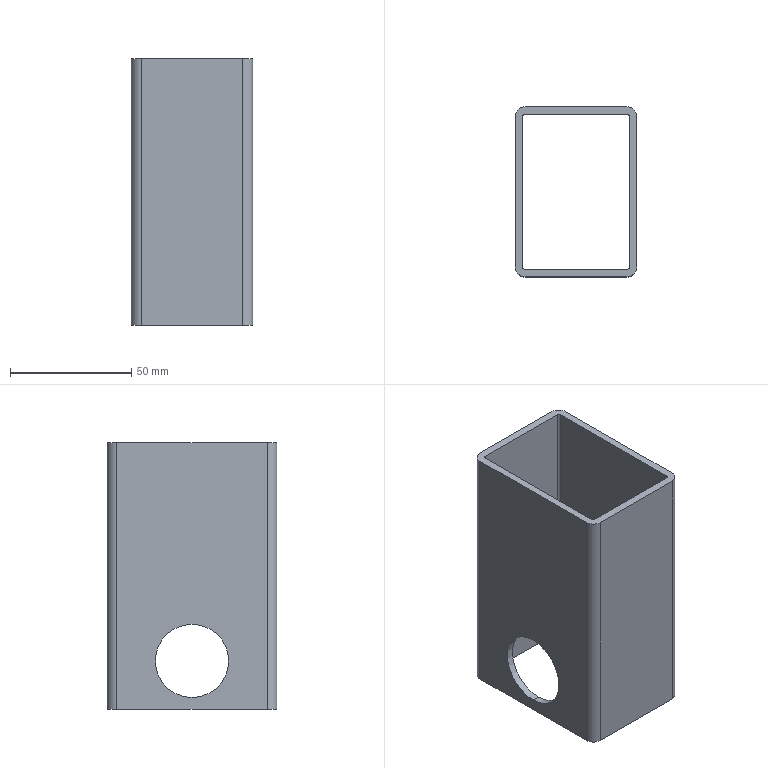Part | SolidWorks | features ExtruThin 1, ICE 1 | 1 solid | 22 faces | box 50 x 70 x 110 mm | volume 69526 mm3 | cylinder 12 | plane 10 | commonest cylinder face diameters 2 x4 8 x4 30.2 x4
STEP:
#1=CARTESIAN_POINT('',(22.,0.,4.9));
#2=VERTEX_POINT('',#1);
#3=CARTESIAN_POINT('',(22.,0.,35.1));
#4=VERTEX_POINT('',#3);
#5=CARTESIAN_POINT('',(22.,0.,20.));
#6=DIRECTION('',(-1.,0.,0.));
#7=DIRECTION('',(0.,0.,1.));
#8=AXIS2_PLACEMENT_3D('',#5,#6,#7);
#9=CIRCLE('',#8,15.1);
#10=EDGE_CURVE('',#2,#4,#9,.T.);
#11=ORIENTED_EDGE('',*,*,#10,.T.);
#12=CARTESIAN_POINT('',(25.,0.,35.1));
#13=VERTEX_POINT('',#12);
#14=CARTESIAN_POINT('',(-25.,0.,35.1));
#15=DIRECTION('',(1.,0.,0.));
#16=VECTOR('',#15,1000.);
#17=LINE('',#14,#16);
#18=EDGE_CURVE('',#4,#13,#17,.T.);
#19=ORIENTED_EDGE('',*,*,#18,.T.);
#20=CARTESIAN_POINT('',(25.,0.,4.9));
#21=VERTEX_POINT('',#20);
#22=CARTESIAN_POINT('',(25.,0.,20.));
#23=DIRECTION('',(1.,0.,0.));
#24=DIRECTION('',(0.,0.,-1.));
#25=AXIS2_PLACEMENT_3D('',#22,#23,#24);
#26=CIRCLE('',#25,15.1);
#27=EDGE_CURVE('',#13,#21,#26,.T.);
#28=ORIENTED_EDGE('',*,*,#27,.T.);
#29=CARTESIAN_POINT('',(-25.,0.,4.9));
#30=DIRECTION('',(1.,0.,0.));
#31=VECTOR('',#30,1000.);
#32=LINE('',#29,#31);
#33=EDGE_CURVE('',#2,#21,#32,.T.);
#34=ORIENTED_EDGE('',*,*,#33,.F.);
#35=EDGE_LOOP('',(#11,#19,#28,#34));
#36=FACE_OUTER_BOUND('',#35,.T.);
#37=CARTESIAN_POINT('',(-25.,0.,20.));
#38=DIRECTION('',(1.,0.,0.));
#39=DIRECTION('',(0.,0.,-1.));
#40=AXIS2_PLACEMENT_3D('',#37,#38,#39);
#41=CYLINDRICAL_SURFACE('',#40,15.1);
#42=ADVANCED_FACE('',(#36),#41,.F.);
#43=CARTESIAN_POINT('',(-25.,0.,35.1));
#44=VERTEX_POINT('',#43);
#45=CARTESIAN_POINT('',(-25.,0.,4.9));
#46=VERTEX_POINT('',#45);
#47=CARTESIAN_POINT('',(-25.,0.,20.));
#48=DIRECTION('',(1.,0.,0.));
#49=DIRECTION('',(0.,0.,-1.));
#50=AXIS2_PLACEMENT_3D('',#47,#48,#49);
#51=CIRCLE('',#50,15.1);
#52=EDGE_CURVE('',#44,#46,#51,.T.);
#53=ORIENTED_EDGE('',*,*,#52,.F.);
#54=CARTESIAN_POINT('',(-22.,0.,35.1));
#55=VERTEX_POINT('',#54);
#56=CARTESIAN_POINT('',(-25.,0.,35.1));
#57=DIRECTION('',(1.,0.,0.));
#58=VECTOR('',#57,1000.);
#59=LINE('',#56,#58);
#60=EDGE_CURVE('',#44,#55,#59,.T.);
#61=ORIENTED_EDGE('',*,*,#60,.T.);
#62=CARTESIAN_POINT('',(-22.,0.,4.9));
#63=VERTEX_POINT('',#62);
#64=CARTESIAN_POINT('',(-22.,0.,20.));
#65=DIRECTION('',(1.,0.,0.));
#66=DIRECTION('',(0.,0.,-1.));
#67=AXIS2_PLACEMENT_3D('',#64,#65,#66);
#68=CIRCLE('',#67,15.1);
#69=EDGE_CURVE('',#55,#63,#68,.T.);
#70=ORIENTED_EDGE('',*,*,#69,.T.);
#71=CARTESIAN_POINT('',(-25.,0.,4.9));
#72=DIRECTION('',(1.,0.,0.));
#73=VECTOR('',#72,1000.);
#74=LINE('',#71,#73);
#75=EDGE_CURVE('',#46,#63,#74,.T.);
#76=ORIENTED_EDGE('',*,*,#75,.F.);
#77=EDGE_LOOP('',(#53,#61,#70,#76));
#78=FACE_OUTER_BOUND('',#77,.T.);
#79=CARTESIAN_POINT('',(-25.,0.,20.));
#80=DIRECTION('',(1.,0.,0.));
#81=DIRECTION('',(0.,0.,-1.));
#82=AXIS2_PLACEMENT_3D('',#79,#80,#81);
#83=CYLINDRICAL_SURFACE('',#82,15.1);
#84=ADVANCED_FACE('',(#78),#83,.F.);
#85=CARTESIAN_POINT('',(-25.,-31.,110.));
#86=VERTEX_POINT('',#85);
#87=CARTESIAN_POINT('',(-21.,-35.,110.));
#88=VERTEX_POINT('',#87);
#89=CARTESIAN_POINT('',(-21.,-31.,110.));
#90=DIRECTION('',(0.,0.,1.));
#91=DIRECTION('',(-1.,0.,0.));
#92=AXIS2_PLACEMENT_3D('',#89,#90,#91);
#93=CIRCLE('',#92,4.);
#94=EDGE_CURVE('',#86,#88,#93,.T.);
#95=ORIENTED_EDGE('',*,*,#94,.T.);
#96=CARTESIAN_POINT('',(21.,-35.,110.));
#97=VERTEX_POINT('',#96);
#98=CARTESIAN_POINT('',(-21.,-35.,110.));
#99=DIRECTION('',(1.,0.,0.));
#100=VECTOR('',#99,1000.);
#101=LINE('',#98,#100);
#102=EDGE_CURVE('',#88,#97,#101,.T.);
#103=ORIENTED_EDGE('',*,*,#102,.T.);
#104=CARTESIAN_POINT('',(25.,-31.,110.));
#105=VERTEX_POINT('',#104);
#106=CARTESIAN_POINT('',(21.,-31.,110.));
#107=DIRECTION('',(0.,0.,1.));
#108=DIRECTION('',(1.,0.,0.));
#109=AXIS2_PLACEMENT_3D('',#106,#107,#108);
#110=CIRCLE('',#109,4.);
#111=EDGE_CURVE('',#97,#105,#110,.T.);
#112=ORIENTED_EDGE('',*,*,#111,.T.);
#113=CARTESIAN_POINT('',(25.,31.,110.));
#114=VERTEX_POINT('',#113);
#115=CARTESIAN_POINT('',(25.,-31.,110.));
#116=DIRECTION('',(0.,1.,0.));
#117=VECTOR('',#116,1000.);
#118=LINE('',#115,#117);
#119=EDGE_CURVE('',#105,#114,#118,.T.);
#120=ORIENTED_EDGE('',*,*,#119,.T.);
#121=CARTESIAN_POINT('',(21.,35.,110.));
#122=VERTEX_POINT('',#121);
#123=CARTESIAN_POINT('',(21.,31.,110.));
#124=DIRECTION('',(0.,0.,1.));
#125=DIRECTION('',(-1.,0.,0.));
#126=AXIS2_PLACEMENT_3D('',#123,#124,#125);
#127=CIRCLE('',#126,4.);
#128=EDGE_CURVE('',#114,#122,#127,.T.);
#129=ORIENTED_EDGE('',*,*,#128,.T.);
#130=CARTESIAN_POINT('',(-21.,35.,110.));
#131=VERTEX_POINT('',#130);
#132=CARTESIAN_POINT('',(-21.,35.,110.));
#133=DIRECTION('',(-1.,0.,0.));
#134=VECTOR('',#133,1000.);
#135=LINE('',#132,#134);
#136=EDGE_CURVE('',#122,#131,#135,.T.);
#137=ORIENTED_EDGE('',*,*,#136,.T.);
#138=CARTESIAN_POINT('',(-25.,31.,110.));
#139=VERTEX_POINT('',#138);
#140=CARTESIAN_POINT('',(-21.,31.,110.));
#141=DIRECTION('',(0.,0.,1.));
#142=DIRECTION('',(-1.,0.,0.));
#143=AXIS2_PLACEMENT_3D('',#140,#141,#142);
#144=CIRCLE('',#143,4.);
#145=EDGE_CURVE('',#131,#139,#144,.T.);
#146=ORIENTED_EDGE('',*,*,#145,.T.);
#147=CARTESIAN_POINT('',(-25.,-31.,110.));
#148=DIRECTION('',(0.,-1.,0.));
#149=VECTOR('',#148,1000.);
#150=LINE('',#147,#149);
#151=EDGE_CURVE('',#139,#86,#150,.T.);
#152=ORIENTED_EDGE('',*,*,#151,.T.);
#153=EDGE_LOOP('',(#95,#103,#112,#120,#129,#137,#146,#152));
#154=FACE_OUTER_BOUND('',#153,.T.);
#155=CARTESIAN_POINT('',(-21.,-32.,110.));
#156=VERTEX_POINT('',#155);
#157=CARTESIAN_POINT('',(21.,-32.,110.));
#158=VERTEX_POINT('',#157);
#159=CARTESIAN_POINT('',(-21.,-32.,110.));
#160=DIRECTION('',(1.,0.,0.));
#161=VECTOR('',#160,1000.);
#162=LINE('',#159,#161);
#163=EDGE_CURVE('',#156,#158,#162,.T.);
#164=ORIENTED_EDGE('',*,*,#163,.F.);
#165=CARTESIAN_POINT('',(-22.,-31.,110.));
#166=VERTEX_POINT('',#165);
#167=CARTESIAN_POINT('',(-21.,-31.,110.));
#168=DIRECTION('',(0.,0.,1.));
#169=DIRECTION('',(-1.,0.,0.));
#170=AXIS2_PLACEMENT_3D('',#167,#168,#169);
#171=CIRCLE('',#170,1.);
#172=EDGE_CURVE('',#166,#156,#171,.T.);
#173=ORIENTED_EDGE('',*,*,#172,.F.);
#174=CARTESIAN_POINT('',(-22.,31.,110.));
#175=VERTEX_POINT('',#174);
#176=CARTESIAN_POINT('',(-22.,-31.,110.));
#177=DIRECTION('',(0.,-1.,0.));
#178=VECTOR('',#177,1000.);
#179=LINE('',#176,#178);
#180=EDGE_CURVE('',#175,#166,#179,.T.);
#181=ORIENTED_EDGE('',*,*,#180,.F.);
#182=CARTESIAN_POINT('',(-21.,32.,110.));
#183=VERTEX_POINT('',#182);
#184=CARTESIAN_POINT('',(-21.,31.,110.));
#185=DIRECTION('',(0.,0.,1.));
#186=DIRECTION('',(-1.,0.,0.));
#187=AXIS2_PLACEMENT_3D('',#184,#185,#186);
#188=CIRCLE('',#187,1.);
#189=EDGE_CURVE('',#183,#175,#188,.T.);
#190=ORIENTED_EDGE('',*,*,#189,.F.);
#191=CARTESIAN_POINT('',(21.,32.,110.));
#192=VERTEX_POINT('',#191);
#193=CARTESIAN_POINT('',(-21.,32.,110.));
#194=DIRECTION('',(-1.,0.,0.));
#195=VECTOR('',#194,1000.);
#196=LINE('',#193,#195);
#197=EDGE_CURVE('',#192,#183,#196,.T.);
#198=ORIENTED_EDGE('',*,*,#197,.F.);
#199=CARTESIAN_POINT('',(22.,31.,110.));
#200=VERTEX_POINT('',#199);
#201=CARTESIAN_POINT('',(21.,31.,110.));
#202=DIRECTION('',(0.,0.,1.));
#203=DIRECTION('',(-1.,0.,0.));
#204=AXIS2_PLACEMENT_3D('',#201,#202,#203);
#205=CIRCLE('',#204,1.);
#206=EDGE_CURVE('',#200,#192,#205,.T.);
#207=ORIENTED_EDGE('',*,*,#206,.F.);
#208=CARTESIAN_POINT('',(22.,-31.,110.));
#209=VERTEX_POINT('',#208);
#210=CARTESIAN_POINT('',(22.,-31.,110.));
#211=DIRECTION('',(0.,1.,0.));
#212=VECTOR('',#211,1000.);
#213=LINE('',#210,#212);
#214=EDGE_CURVE('',#209,#200,#213,.T.);
#215=ORIENTED_EDGE('',*,*,#214,.F.);
#216=CARTESIAN_POINT('',(21.,-31.,110.));
#217=DIRECTION('',(0.,0.,1.));
#218=DIRECTION('',(-1.,0.,0.));
#219=AXIS2_PLACEMENT_3D('',#216,#217,#218);
#220=CIRCLE('',#219,1.);
#221=EDGE_CURVE('',#158,#209,#220,.T.);
#222=ORIENTED_EDGE('',*,*,#221,.F.);
#223=EDGE_LOOP('',(#164,#173,#181,#190,#198,#207,#215,#222));
#224=FACE_BOUND('',#223,.T.);
#225=CARTESIAN_POINT('',(-21.,-31.,110.));
#226=DIRECTION('',(0.,0.,1.));
#227=DIRECTION('',(1.,0.,0.));
#228=AXIS2_PLACEMENT_3D('',#225,#226,#227);
#229=PLANE('',#228);
#230=ADVANCED_FACE('',(#154,#224),#229,.T.);
#231=CARTESIAN_POINT('',(-25.,-31.,0.));
#232=VERTEX_POINT('',#231);
#233=CARTESIAN_POINT('',(-21.,-35.,0.));
#234=VERTEX_POINT('',#233);
#235=CARTESIAN_POINT('',(-21.,-31.,0.));
#236=DIRECTION('',(0.,0.,1.));
#237=DIRECTION('',(-1.,0.,0.));
#238=AXIS2_PLACEMENT_3D('',#235,#236,#237);
#239=CIRCLE('',#238,4.);
#240=EDGE_CURVE('',#232,#234,#239,.T.);
#241=ORIENTED_EDGE('',*,*,#240,.F.);
#242=CARTESIAN_POINT('',(-25.,31.,0.));
#243=VERTEX_POINT('',#242);
#244=CARTESIAN_POINT('',(-25.,-31.,0.));
#245=DIRECTION('',(0.,-1.,0.));
#246=VECTOR('',#245,1000.);
#247=LINE('',#244,#246);
#248=EDGE_CURVE('',#243,#232,#247,.T.);
#249=ORIENTED_EDGE('',*,*,#248,.F.);
#250=CARTESIAN_POINT('',(-21.,35.,0.));
#251=VERTEX_POINT('',#250);
#252=CARTESIAN_POINT('',(-21.,31.,0.));
#253=DIRECTION('',(0.,0.,1.));
#254=DIRECTION('',(-1.,0.,0.));
#255=AXIS2_PLACEMENT_3D('',#252,#253,#254);
#256=CIRCLE('',#255,4.);
#257=EDGE_CURVE('',#251,#243,#256,.T.);
#258=ORIENTED_EDGE('',*,*,#257,.F.);
#259=CARTESIAN_POINT('',(21.,35.,0.));
#260=VERTEX_POINT('',#259);
#261=CARTESIAN_POINT('',(-21.,35.,0.));
#262=DIRECTION('',(-1.,0.,0.));
#263=VECTOR('',#262,1000.);
#264=LINE('',#261,#263);
#265=EDGE_CURVE('',#260,#251,#264,.T.);
#266=ORIENTED_EDGE('',*,*,#265,.F.);
#267=CARTESIAN_POINT('',(25.,31.,0.));
#268=VERTEX_POINT('',#267);
#269=CARTESIAN_POINT('',(21.,31.,0.));
#270=DIRECTION('',(0.,0.,1.));
#271=DIRECTION('',(-1.,0.,0.));
#272=AXIS2_PLACEMENT_3D('',#269,#270,#271);
#273=CIRCLE('',#272,4.);
#274=EDGE_CURVE('',#268,#260,#273,.T.);
#275=ORIENTED_EDGE('',*,*,#274,.F.);
#276=CARTESIAN_POINT('',(25.,-31.,0.));
#277=VERTEX_POINT('',#276);
#278=CARTESIAN_POINT('',(25.,-31.,0.));
#279=DIRECTION('',(0.,1.,0.));
#280=VECTOR('',#279,1000.);
#281=LINE('',#278,#280);
#282=EDGE_CURVE('',#277,#268,#281,.T.);
#283=ORIENTED_EDGE('',*,*,#282,.F.);
#284=CARTESIAN_POINT('',(21.,-35.,0.));
#285=VERTEX_POINT('',#284);
#286=CARTESIAN_POINT('',(21.,-31.,0.));
#287=DIRECTION('',(0.,0.,1.));
#288=DIRECTION('',(1.,0.,0.));
#289=AXIS2_PLACEMENT_3D('',#286,#287,#288);
#290=CIRCLE('',#289,4.);
#291=EDGE_CURVE('',#285,#277,#290,.T.);
#292=ORIENTED_EDGE('',*,*,#291,.F.);
#293=CARTESIAN_POINT('',(-21.,-35.,0.));
#294=DIRECTION('',(1.,0.,0.));
#295=VECTOR('',#294,1000.);
#296=LINE('',#293,#295);
#297=EDGE_CURVE('',#234,#285,#296,.T.);
#298=ORIENTED_EDGE('',*,*,#297,.F.);
#299=EDGE_LOOP('',(#241,#249,#258,#266,#275,#283,#292,#298));
#300=FACE_OUTER_BOUND('',#299,.T.);
#301=CARTESIAN_POINT('',(-22.,-31.,0.));
#302=VERTEX_POINT('',#301);
#303=CARTESIAN_POINT('',(-21.,-32.,0.));
#304=VERTEX_POINT('',#303);
#305=CARTESIAN_POINT('',(-21.,-31.,0.));
#306=DIRECTION('',(0.,0.,1.));
#307=DIRECTION('',(-1.,0.,0.));
#308=AXIS2_PLACEMENT_3D('',#305,#306,#307);
#309=CIRCLE('',#308,1.);
#310=EDGE_CURVE('',#302,#304,#309,.T.);
#311=ORIENTED_EDGE('',*,*,#310,.T.);
#312=CARTESIAN_POINT('',(21.,-32.,0.));
#313=VERTEX_POINT('',#312);
#314=CARTESIAN_POINT('',(-21.,-32.,0.));
#315=DIRECTION('',(1.,0.,0.));
#316=VECTOR('',#315,1000.);
#317=LINE('',#314,#316);
#318=EDGE_CURVE('',#304,#313,#317,.T.);
#319=ORIENTED_EDGE('',*,*,#318,.T.);
#320=CARTESIAN_POINT('',(22.,-31.,0.));
#321=VERTEX_POINT('',#320);
#322=CARTESIAN_POINT('',(21.,-31.,0.));
#323=DIRECTION('',(0.,0.,1.));
#324=DIRECTION('',(-1.,0.,0.));
#325=AXIS2_PLACEMENT_3D('',#322,#323,#324);
#326=CIRCLE('',#325,1.);
#327=EDGE_CURVE('',#313,#321,#326,.T.);
#328=ORIENTED_EDGE('',*,*,#327,.T.);
#329=CARTESIAN_POINT('',(22.,31.,0.));
#330=VERTEX_POINT('',#329);
#331=CARTESIAN_POINT('',(22.,-31.,0.));
#332=DIRECTION('',(0.,1.,0.));
#333=VECTOR('',#332,1000.);
#334=LINE('',#331,#333);
#335=EDGE_CURVE('',#321,#330,#334,.T.);
#336=ORIENTED_EDGE('',*,*,#335,.T.);
#337=CARTESIAN_POINT('',(21.,32.,0.));
#338=VERTEX_POINT('',#337);
#339=CARTESIAN_POINT('',(21.,31.,0.));
#340=DIRECTION('',(0.,0.,1.));
#341=DIRECTION('',(-1.,0.,0.));
#342=AXIS2_PLACEMENT_3D('',#339,#340,#341);
#343=CIRCLE('',#342,1.);
#344=EDGE_CURVE('',#330,#338,#343,.T.);
#345=ORIENTED_EDGE('',*,*,#344,.T.);
#346=CARTESIAN_POINT('',(-21.,32.,0.));
#347=VERTEX_POINT('',#346);
#348=CARTESIAN_POINT('',(-21.,32.,0.));
#349=DIRECTION('',(-1.,0.,0.));
#350=VECTOR('',#349,1000.);
#351=LINE('',#348,#350);
#352=EDGE_CURVE('',#338,#347,#351,.T.);
#353=ORIENTED_EDGE('',*,*,#352,.T.);
#354=CARTESIAN_POINT('',(-22.,31.,0.));
#355=VERTEX_POINT('',#354);
#356=CARTESIAN_POINT('',(-21.,31.,0.));
#357=DIRECTION('',(0.,0.,1.));
#358=DIRECTION('',(-1.,0.,0.));
#359=AXIS2_PLACEMENT_3D('',#356,#357,#358);
#360=CIRCLE('',#359,1.);
#361=EDGE_CURVE('',#347,#355,#360,.T.);
#362=ORIENTED_EDGE('',*,*,#361,.T.);
#363=CARTESIAN_POINT('',(-22.,-31.,0.));
#364=DIRECTION('',(0.,-1.,0.));
#365=VECTOR('',#364,1000.);
#366=LINE('',#363,#365);
#367=EDGE_CURVE('',#355,#302,#366,.T.);
#368=ORIENTED_EDGE('',*,*,#367,.T.);
#369=EDGE_LOOP('',(#311,#319,#328,#336,#345,#353,#362,#368));
#370=FACE_BOUND('',#369,.T.);
#371=CARTESIAN_POINT('',(-21.,-31.,0.));
#372=DIRECTION('',(0.,0.,1.));
#373=DIRECTION('',(1.,0.,0.));
#374=AXIS2_PLACEMENT_3D('',#371,#372,#373);
#375=PLANE('',#374);
#376=ADVANCED_FACE('',(#300,#370),#375,.F.);
#377=ORIENTED_EDGE('',*,*,#240,.T.);
#378=CARTESIAN_POINT('',(-21.,-35.,110.));
#379=DIRECTION('',(0.,0.,-1.));
#380=VECTOR('',#379,1000.);
#381=LINE('',#378,#380);
#382=EDGE_CURVE('',#88,#234,#381,.T.);
#383=ORIENTED_EDGE('',*,*,#382,.F.);
#384=ORIENTED_EDGE('',*,*,#94,.F.);
#385=CARTESIAN_POINT('',(-25.,-31.,110.));
#386=DIRECTION('',(0.,0.,-1.));
#387=VECTOR('',#386,1000.);
#388=LINE('',#385,#387);
#389=EDGE_CURVE('',#86,#232,#388,.T.);
#390=ORIENTED_EDGE('',*,*,#389,.T.);
#391=EDGE_LOOP('',(#377,#383,#384,#390));
#392=FACE_OUTER_BOUND('',#391,.T.);
#393=CARTESIAN_POINT('',(-21.,-31.,110.));
#394=DIRECTION('',(0.,0.,-1.));
#395=DIRECTION('',(-1.,0.,0.));
#396=AXIS2_PLACEMENT_3D('',#393,#394,#395);
#397=CYLINDRICAL_SURFACE('',#396,4.);
#398=ADVANCED_FACE('',(#392),#397,.T.);
#399=ORIENTED_EDGE('',*,*,#297,.T.);
#400=CARTESIAN_POINT('',(21.,-35.,110.));
#401=DIRECTION('',(0.,0.,-1.));
#402=VECTOR('',#401,1000.);
#403=LINE('',#400,#402);
#404=EDGE_CURVE('',#97,#285,#403,.T.);
#405=ORIENTED_EDGE('',*,*,#404,.F.);
#406=ORIENTED_EDGE('',*,*,#102,.F.);
#407=ORIENTED_EDGE('',*,*,#382,.T.);
#408=EDGE_LOOP('',(#399,#405,#406,#407));
#409=FACE_OUTER_BOUND('',#408,.T.);
#410=CARTESIAN_POINT('',(-21.,-35.,110.));
#411=DIRECTION('',(0.,1.,0.));
#412=DIRECTION('',(0.,0.,1.));
#413=AXIS2_PLACEMENT_3D('',#410,#411,#412);
#414=PLANE('',#413);
#415=ADVANCED_FACE('',(#409),#414,.F.);
#416=ORIENTED_EDGE('',*,*,#291,.T.);
#417=CARTESIAN_POINT('',(25.,-31.,110.));
#418=DIRECTION('',(0.,0.,-1.));
#419=VECTOR('',#418,1000.);
#420=LINE('',#417,#419);
#421=EDGE_CURVE('',#105,#277,#420,.T.);
#422=ORIENTED_EDGE('',*,*,#421,.F.);
#423=ORIENTED_EDGE('',*,*,#111,.F.);
#424=ORIENTED_EDGE('',*,*,#404,.T.);
#425=EDGE_LOOP('',(#416,#422,#423,#424));
#426=FACE_OUTER_BOUND('',#425,.T.);
#427=CARTESIAN_POINT('',(21.,-31.,110.));
#428=DIRECTION('',(0.,0.,-1.));
#429=DIRECTION('',(-1.,0.,0.));
#430=AXIS2_PLACEMENT_3D('',#427,#428,#429);
#431=CYLINDRICAL_SURFACE('',#430,4.);
#432=ADVANCED_FACE('',(#426),#431,.T.);
#433=CARTESIAN_POINT('',(25.,0.,20.));
#434=DIRECTION('',(1.,0.,0.));
#435=DIRECTION('',(0.,0.,-1.));
#436=AXIS2_PLACEMENT_3D('',#433,#434,#435);
#437=CIRCLE('',#436,15.1);
#438=EDGE_CURVE('',#21,#13,#437,.T.);
#439=ORIENTED_EDGE('',*,*,#438,.F.);
#440=ORIENTED_EDGE('',*,*,#27,.F.);
#441=EDGE_LOOP('',(#439,#440));
#442=FACE_BOUND('',#441,.T.);
#443=ORIENTED_EDGE('',*,*,#282,.T.);
#444=CARTESIAN_POINT('',(25.,31.,110.));
#445=DIRECTION('',(0.,0.,-1.));
#446=VECTOR('',#445,1000.);
#447=LINE('',#444,#446);
#448=EDGE_CURVE('',#114,#268,#447,.T.);
#449=ORIENTED_EDGE('',*,*,#448,.F.);
#450=ORIENTED_EDGE('',*,*,#119,.F.);
#451=ORIENTED_EDGE('',*,*,#421,.T.);
#452=EDGE_LOOP('',(#443,#449,#450,#451));
#453=FACE_OUTER_BOUND('',#452,.T.);
#454=CARTESIAN_POINT('',(25.,-31.,110.));
#455=DIRECTION('',(-1.,0.,0.));
#456=DIRECTION('',(0.,0.,1.));
#457=AXIS2_PLACEMENT_3D('',#454,#455,#456);
#458=PLANE('',#457);
#459=ADVANCED_FACE('',(#442,#453),#458,.F.);
#460=ORIENTED_EDGE('',*,*,#274,.T.);
#461=CARTESIAN_POINT('',(21.,35.,110.));
#462=DIRECTION('',(0.,0.,-1.));
#463=VECTOR('',#462,1000.);
#464=LINE('',#461,#463);
#465=EDGE_CURVE('',#122,#260,#464,.T.);
#466=ORIENTED_EDGE('',*,*,#465,.F.);
#467=ORIENTED_EDGE('',*,*,#128,.F.);
#468=ORIENTED_EDGE('',*,*,#448,.T.);
#469=EDGE_LOOP('',(#460,#466,#467,#468));
#470=FACE_OUTER_BOUND('',#469,.T.);
#471=CARTESIAN_POINT('',(21.,31.,110.));
#472=DIRECTION('',(0.,0.,-1.));
#473=DIRECTION('',(-1.,0.,0.));
#474=AXIS2_PLACEMENT_3D('',#471,#472,#473);
#475=CYLINDRICAL_SURFACE('',#474,4.);
#476=ADVANCED_FACE('',(#470),#475,.T.);
#477=ORIENTED_EDGE('',*,*,#265,.T.);
#478=CARTESIAN_POINT('',(-21.,35.,110.));
#479=DIRECTION('',(0.,0.,-1.));
#480=VECTOR('',#479,1000.);
#481=LINE('',#478,#480);
#482=EDGE_CURVE('',#131,#251,#481,.T.);
#483=ORIENTED_EDGE('',*,*,#482,.F.);
#484=ORIENTED_EDGE('',*,*,#136,.F.);
#485=ORIENTED_EDGE('',*,*,#465,.T.);
#486=EDGE_LOOP('',(#477,#483,#484,#485));
#487=FACE_OUTER_BOUND('',#486,.T.);
#488=CARTESIAN_POINT('',(-21.,35.,110.));
#489=DIRECTION('',(0.,-1.,0.));
#490=DIRECTION('',(0.,0.,-1.));
#491=AXIS2_PLACEMENT_3D('',#488,#489,#490);
#492=PLANE('',#491);
#493=ADVANCED_FACE('',(#487),#492,.F.);
#494=ORIENTED_EDGE('',*,*,#257,.T.);
#495=CARTESIAN_POINT('',(-25.,31.,110.));
#496=DIRECTION('',(0.,0.,-1.));
#497=VECTOR('',#496,1000.);
#498=LINE('',#495,#497);
#499=EDGE_CURVE('',#139,#243,#498,.T.);
#500=ORIENTED_EDGE('',*,*,#499,.F.);
#501=ORIENTED_EDGE('',*,*,#145,.F.);
#502=ORIENTED_EDGE('',*,*,#482,.T.);
#503=EDGE_LOOP('',(#494,#500,#501,#502));
#504=FACE_OUTER_BOUND('',#503,.T.);
#505=CARTESIAN_POINT('',(-21.,31.,110.));
#506=DIRECTION('',(0.,0.,-1.));
#507=DIRECTION('',(-1.,0.,0.));
#508=AXIS2_PLACEMENT_3D('',#505,#506,#507);
#509=CYLINDRICAL_SURFACE('',#508,4.);
#510=ADVANCED_FACE('',(#504),#509,.T.);
#511=CARTESIAN_POINT('',(-25.,0.,20.));
#512=DIRECTION('',(1.,0.,0.));
#513=DIRECTION('',(0.,0.,-1.));
#514=AXIS2_PLACEMENT_3D('',#511,#512,#513);
#515=CIRCLE('',#514,15.1);
#516=EDGE_CURVE('',#46,#44,#515,.T.);
#517=ORIENTED_EDGE('',*,*,#516,.T.);
#518=ORIENTED_EDGE('',*,*,#52,.T.);
#519=EDGE_LOOP('',(#517,#518));
#520=FACE_BOUND('',#519,.T.);
#521=ORIENTED_EDGE('',*,*,#248,.T.);
#522=ORIENTED_EDGE('',*,*,#389,.F.);
#523=ORIENTED_EDGE('',*,*,#151,.F.);
#524=ORIENTED_EDGE('',*,*,#499,.T.);
#525=EDGE_LOOP('',(#521,#522,#523,#524));
#526=FACE_OUTER_BOUND('',#525,.T.);
#527=CARTESIAN_POINT('',(-25.,-31.,110.));
#528=DIRECTION('',(1.,0.,0.));
#529=DIRECTION('',(0.,0.,-1.));
#530=AXIS2_PLACEMENT_3D('',#527,#528,#529);
#531=PLANE('',#530);
#532=ADVANCED_FACE('',(#520,#526),#531,.F.);
#533=ORIENTED_EDGE('',*,*,#310,.F.);
#534=CARTESIAN_POINT('',(-22.,-31.,110.));
#535=DIRECTION('',(0.,0.,-1.));
#536=VECTOR('',#535,1000.);
#537=LINE('',#534,#536);
#538=EDGE_CURVE('',#166,#302,#537,.T.);
#539=ORIENTED_EDGE('',*,*,#538,.F.);
#540=ORIENTED_EDGE('',*,*,#172,.T.);
#541=CARTESIAN_POINT('',(-21.,-32.,110.));
#542=DIRECTION('',(0.,0.,-1.));
#543=VECTOR('',#542,1000.);
#544=LINE('',#541,#543);
#545=EDGE_CURVE('',#156,#304,#544,.T.);
#546=ORIENTED_EDGE('',*,*,#545,.T.);
#547=EDGE_LOOP('',(#533,#539,#540,#546));
#548=FACE_OUTER_BOUND('',#547,.T.);
#549=CARTESIAN_POINT('',(-21.,-31.,110.));
#550=DIRECTION('',(0.,0.,-1.));
#551=DIRECTION('',(-1.,0.,0.));
#552=AXIS2_PLACEMENT_3D('',#549,#550,#551);
#553=CYLINDRICAL_SURFACE('',#552,1.);
#554=ADVANCED_FACE('',(#548),#553,.F.);
#555=ORIENTED_EDGE('',*,*,#318,.F.);
#556=ORIENTED_EDGE('',*,*,#545,.F.);
#557=ORIENTED_EDGE('',*,*,#163,.T.);
#558=CARTESIAN_POINT('',(21.,-32.,110.));
#559=DIRECTION('',(0.,0.,-1.));
#560=VECTOR('',#559,1000.);
#561=LINE('',#558,#560);
#562=EDGE_CURVE('',#158,#313,#561,.T.);
#563=ORIENTED_EDGE('',*,*,#562,.T.);
#564=EDGE_LOOP('',(#555,#556,#557,#563));
#565=FACE_OUTER_BOUND('',#564,.T.);
#566=CARTESIAN_POINT('',(-21.,-32.,110.));
#567=DIRECTION('',(0.,1.,0.));
#568=DIRECTION('',(0.,0.,1.));
#569=AXIS2_PLACEMENT_3D('',#566,#567,#568);
#570=PLANE('',#569);
#571=ADVANCED_FACE('',(#565),#570,.T.);
#572=ORIENTED_EDGE('',*,*,#327,.F.);
#573=ORIENTED_EDGE('',*,*,#562,.F.);
#574=ORIENTED_EDGE('',*,*,#221,.T.);
#575=CARTESIAN_POINT('',(22.,-31.,110.));
#576=DIRECTION('',(0.,0.,-1.));
#577=VECTOR('',#576,1000.);
#578=LINE('',#575,#577);
#579=EDGE_CURVE('',#209,#321,#578,.T.);
#580=ORIENTED_EDGE('',*,*,#579,.T.);
#581=EDGE_LOOP('',(#572,#573,#574,#580));
#582=FACE_OUTER_BOUND('',#581,.T.);
#583=CARTESIAN_POINT('',(21.,-31.,110.));
#584=DIRECTION('',(0.,0.,-1.));
#585=DIRECTION('',(-1.,0.,0.));
#586=AXIS2_PLACEMENT_3D('',#583,#584,#585);
#587=CYLINDRICAL_SURFACE('',#586,1.);
#588=ADVANCED_FACE('',(#582),#587,.F.);
#589=ORIENTED_EDGE('',*,*,#10,.F.);
#590=CARTESIAN_POINT('',(22.,0.,20.));
#591=DIRECTION('',(-1.,0.,0.));
#592=DIRECTION('',(0.,0.,1.));
#593=AXIS2_PLACEMENT_3D('',#590,#591,#592);
#594=CIRCLE('',#593,15.1);
#595=EDGE_CURVE('',#4,#2,#594,.T.);
#596=ORIENTED_EDGE('',*,*,#595,.F.);
#597=EDGE_LOOP('',(#589,#596));
#598=FACE_BOUND('',#597,.T.);
#599=ORIENTED_EDGE('',*,*,#335,.F.);
#600=ORIENTED_EDGE('',*,*,#579,.F.);
#601=ORIENTED_EDGE('',*,*,#214,.T.);
#602=CARTESIAN_POINT('',(22.,31.,110.));
#603=DIRECTION('',(0.,0.,-1.));
#604=VECTOR('',#603,1000.);
#605=LINE('',#602,#604);
#606=EDGE_CURVE('',#200,#330,#605,.T.);
#607=ORIENTED_EDGE('',*,*,#606,.T.);
#608=EDGE_LOOP('',(#599,#600,#601,#607));
#609=FACE_OUTER_BOUND('',#608,.T.);
#610=CARTESIAN_POINT('',(22.,-31.,110.));
#611=DIRECTION('',(-1.,0.,0.));
#612=DIRECTION('',(0.,0.,1.));
#613=AXIS2_PLACEMENT_3D('',#610,#611,#612);
#614=PLANE('',#613);
#615=ADVANCED_FACE('',(#598,#609),#614,.T.);
#616=ORIENTED_EDGE('',*,*,#344,.F.);
#617=ORIENTED_EDGE('',*,*,#606,.F.);
#618=ORIENTED_EDGE('',*,*,#206,.T.);
#619=CARTESIAN_POINT('',(21.,32.,110.));
#620=DIRECTION('',(0.,0.,-1.));
#621=VECTOR('',#620,1000.);
#622=LINE('',#619,#621);
#623=EDGE_CURVE('',#192,#338,#622,.T.);
#624=ORIENTED_EDGE('',*,*,#623,.T.);
#625=EDGE_LOOP('',(#616,#617,#618,#624));
#626=FACE_OUTER_BOUND('',#625,.T.);
#627=CARTESIAN_POINT('',(21.,31.,110.));
#628=DIRECTION('',(0.,0.,-1.));
#629=DIRECTION('',(-1.,0.,0.));
#630=AXIS2_PLACEMENT_3D('',#627,#628,#629);
#631=CYLINDRICAL_SURFACE('',#630,1.);
#632=ADVANCED_FACE('',(#626),#631,.F.);
#633=ORIENTED_EDGE('',*,*,#352,.F.);
#634=ORIENTED_EDGE('',*,*,#623,.F.);
#635=ORIENTED_EDGE('',*,*,#197,.T.);
#636=CARTESIAN_POINT('',(-21.,32.,110.));
#637=DIRECTION('',(0.,0.,-1.));
#638=VECTOR('',#637,1000.);
#639=LINE('',#636,#638);
#640=EDGE_CURVE('',#183,#347,#639,.T.);
#641=ORIENTED_EDGE('',*,*,#640,.T.);
#642=EDGE_LOOP('',(#633,#634,#635,#641));
#643=FACE_OUTER_BOUND('',#642,.T.);
#644=CARTESIAN_POINT('',(-21.,32.,110.));
#645=DIRECTION('',(0.,-1.,0.));
#646=DIRECTION('',(0.,0.,-1.));
#647=AXIS2_PLACEMENT_3D('',#644,#645,#646);
#648=PLANE('',#647);
#649=ADVANCED_FACE('',(#643),#648,.T.);
#650=ORIENTED_EDGE('',*,*,#361,.F.);
#651=ORIENTED_EDGE('',*,*,#640,.F.);
#652=ORIENTED_EDGE('',*,*,#189,.T.);
#653=CARTESIAN_POINT('',(-22.,31.,110.));
#654=DIRECTION('',(0.,0.,-1.));
#655=VECTOR('',#654,1000.);
#656=LINE('',#653,#655);
#657=EDGE_CURVE('',#175,#355,#656,.T.);
#658=ORIENTED_EDGE('',*,*,#657,.T.);
#659=EDGE_LOOP('',(#650,#651,#652,#658));
#660=FACE_OUTER_BOUND('',#659,.T.);
#661=CARTESIAN_POINT('',(-21.,31.,110.));
#662=DIRECTION('',(0.,0.,-1.));
#663=DIRECTION('',(-1.,0.,0.));
#664=AXIS2_PLACEMENT_3D('',#661,#662,#663);
#665=CYLINDRICAL_SURFACE('',#664,1.);
#666=ADVANCED_FACE('',(#660),#665,.F.);
#667=CARTESIAN_POINT('',(-22.,0.,20.));
#668=DIRECTION('',(1.,0.,0.));
#669=DIRECTION('',(0.,0.,-1.));
#670=AXIS2_PLACEMENT_3D('',#667,#668,#669);
#671=CIRCLE('',#670,15.1);
#672=EDGE_CURVE('',#63,#55,#671,.T.);
#673=ORIENTED_EDGE('',*,*,#672,.F.);
#674=ORIENTED_EDGE('',*,*,#69,.F.);
#675=EDGE_LOOP('',(#673,#674));
#676=FACE_BOUND('',#675,.T.);
#677=ORIENTED_EDGE('',*,*,#367,.F.);
#678=ORIENTED_EDGE('',*,*,#657,.F.);
#679=ORIENTED_EDGE('',*,*,#180,.T.);
#680=ORIENTED_EDGE('',*,*,#538,.T.);
#681=EDGE_LOOP('',(#677,#678,#679,#680));
#682=FACE_OUTER_BOUND('',#681,.T.);
#683=CARTESIAN_POINT('',(-22.,-31.,110.));
#684=DIRECTION('',(1.,0.,0.));
#685=DIRECTION('',(0.,0.,-1.));
#686=AXIS2_PLACEMENT_3D('',#683,#684,#685);
#687=PLANE('',#686);
#688=ADVANCED_FACE('',(#676,#682),#687,.T.);
#689=ORIENTED_EDGE('',*,*,#60,.F.);
#690=ORIENTED_EDGE('',*,*,#516,.F.);
#691=ORIENTED_EDGE('',*,*,#75,.T.);
#692=ORIENTED_EDGE('',*,*,#672,.T.);
#693=EDGE_LOOP('',(#689,#690,#691,#692));
#694=FACE_OUTER_BOUND('',#693,.T.);
#695=CARTESIAN_POINT('',(-25.,0.,20.));
#696=DIRECTION('',(1.,0.,0.));
#697=DIRECTION('',(0.,0.,-1.));
#698=AXIS2_PLACEMENT_3D('',#695,#696,#697);
#699=CYLINDRICAL_SURFACE('',#698,15.1);
#700=ADVANCED_FACE('',(#694),#699,.F.);
#701=ORIENTED_EDGE('',*,*,#18,.F.);
#702=ORIENTED_EDGE('',*,*,#595,.T.);
#703=ORIENTED_EDGE('',*,*,#33,.T.);
#704=ORIENTED_EDGE('',*,*,#438,.T.);
#705=EDGE_LOOP('',(#701,#702,#703,#704));
#706=FACE_OUTER_BOUND('',#705,.T.);
#707=CARTESIAN_POINT('',(-25.,0.,20.));
#708=DIRECTION('',(1.,0.,0.));
#709=DIRECTION('',(0.,0.,-1.));
#710=AXIS2_PLACEMENT_3D('',#707,#708,#709);
#711=CYLINDRICAL_SURFACE('',#710,15.1);
#712=ADVANCED_FACE('',(#706),#711,.F.);
#713=CLOSED_SHELL('',(#42,#84,#230,#376,#398,#415,#432,#459,#476,#493,#510,#532,#554,#571,#588,#615,#632,#649,#666,#688,#700,#712));
#714=MANIFOLD_SOLID_BREP('',#713);
#715=CARTESIAN_POINT('',(0.,0.,0.));
#716=DIRECTION('',(0.,0.,1.));
#717=DIRECTION('',(1.,0.,0.));
#718=AXIS2_PLACEMENT_3D('',#715,#716,#717);
#719=(LENGTH_UNIT()NAMED_UNIT(*)SI_UNIT(.MILLI.,.METRE.));
#720=UNCERTAINTY_MEASURE_WITH_UNIT(LENGTH_MEASURE(0.00001),#719,'','');
#721=(NAMED_UNIT(*)PLANE_ANGLE_UNIT()SI_UNIT($,.RADIAN.));
#722=(NAMED_UNIT(*)SI_UNIT($,.STERADIAN.)SOLID_ANGLE_UNIT());
#723=(GEOMETRIC_REPRESENTATION_CONTEXT(3)GLOBAL_UNCERTAINTY_ASSIGNED_CONTEXT((#720))GLOBAL_UNIT_ASSIGNED_CONTEXT((#719,#721,#722))REPRESENTATION_CONTEXT('',''));
#724=ADVANCED_BREP_SHAPE_REPRESENTATION('',(#714,#718),#723);